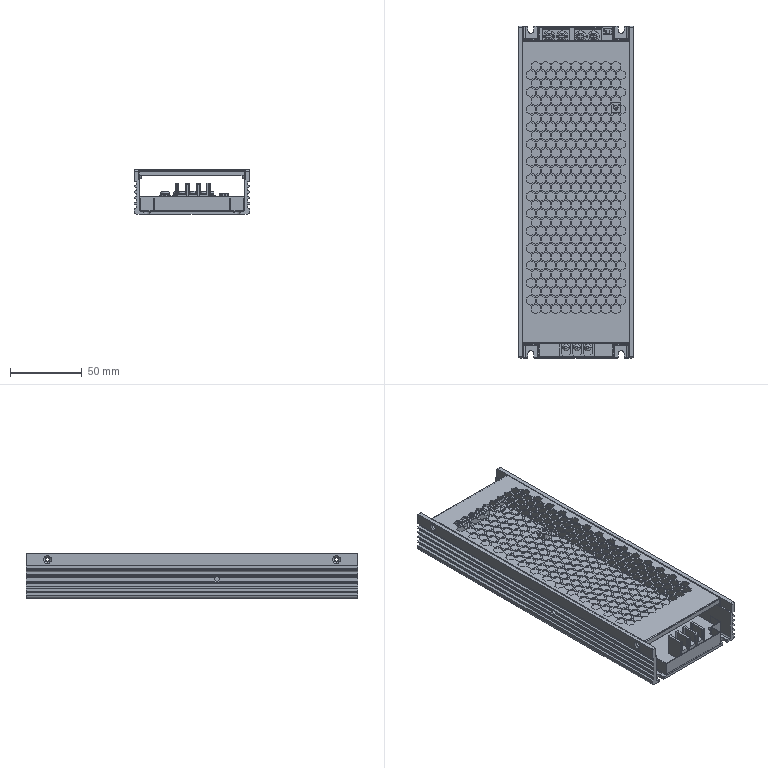Part | STEP file | Power module UHP-500(R) | 18 solids | 2353 faces | box 81 x 232 x 31 mm | volume 117475 mm3 | plane 2107 | cylinder 198 | torus 24 | cone 18 | spline 6 | commonest cylinder face diameters 1 x38 2 x20 2.6 x16 3.5 x16 3.8 x16 6 x16